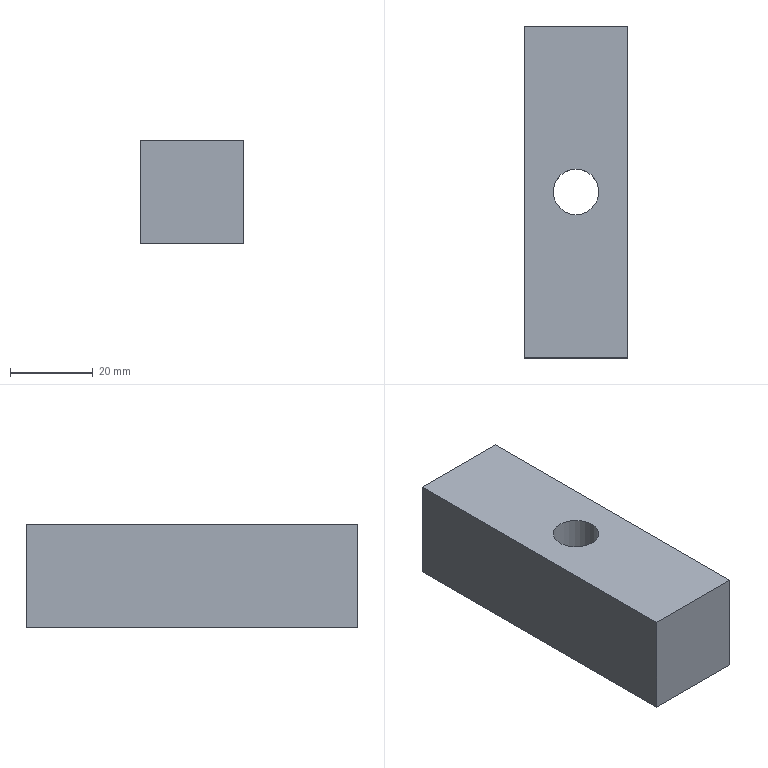Part | NX | features solid 2 | 1 solid | 9 faces | box 25 x 80 x 25 mm | volume 45711 mm3 | plane 7 | cylinder 2 | commonest cylinder face diameters 11 x1 18 x1
STEP:
#1=CARTESIAN_POINT('',(-317.5,-542.5,143.));
#2=VERTEX_POINT('',#1);
#3=CARTESIAN_POINT('',(-317.5,-542.5,118.));
#4=VERTEX_POINT('',#3);
#5=CARTESIAN_POINT('',(-317.5,-542.5,143.));
#6=DIRECTION('',(0.,0.,1.));
#7=VECTOR('',#6,1000.);
#8=LINE('',#5,#7);
#9=EDGE_CURVE('',#2,#4,#8,.F.);
#10=ORIENTED_EDGE('',*,*,#9,.T.);
#11=CARTESIAN_POINT('',(-292.5,-542.5,118.));
#12=VERTEX_POINT('',#11);
#13=CARTESIAN_POINT('',(-317.5,-542.5,118.));
#14=DIRECTION('',(1.,0.,0.));
#15=VECTOR('',#14,1000.);
#16=LINE('',#13,#15);
#17=EDGE_CURVE('',#4,#12,#16,.T.);
#18=ORIENTED_EDGE('',*,*,#17,.T.);
#19=CARTESIAN_POINT('',(-292.5,-542.5,143.));
#20=VERTEX_POINT('',#19);
#21=CARTESIAN_POINT('',(-292.5,-542.5,143.));
#22=DIRECTION('',(0.,0.,-1.));
#23=VECTOR('',#22,1000.);
#24=LINE('',#21,#23);
#25=EDGE_CURVE('',#20,#12,#24,.T.);
#26=ORIENTED_EDGE('',*,*,#25,.F.);
#27=CARTESIAN_POINT('',(-317.5,-542.5,143.));
#28=DIRECTION('',(1.,0.,0.));
#29=VECTOR('',#28,1000.);
#30=LINE('',#27,#29);
#31=EDGE_CURVE('',#2,#20,#30,.T.);
#32=ORIENTED_EDGE('',*,*,#31,.F.);
#33=EDGE_LOOP('',(#10,#18,#26,#32));
#34=FACE_BOUND('',#33,.T.);
#35=CARTESIAN_POINT('',(-317.5,-542.5,143.));
#36=DIRECTION('',(0.,-1.,0.));
#37=DIRECTION('',(1.,0.,0.));
#38=AXIS2_PLACEMENT_3D('',#35,#36,#37);
#39=PLANE('',#38);
#40=ADVANCED_FACE('',(#34),#39,.T.);
#41=ORIENTED_EDGE('',*,*,#25,.T.);
#42=CARTESIAN_POINT('',(-292.5,-462.5,118.));
#43=VERTEX_POINT('',#42);
#44=CARTESIAN_POINT('',(-292.5,-539.5,118.));
#45=DIRECTION('',(0.,-1.,0.));
#46=VECTOR('',#45,1000.);
#47=LINE('',#44,#46);
#48=EDGE_CURVE('',#12,#43,#47,.F.);
#49=ORIENTED_EDGE('',*,*,#48,.T.);
#50=CARTESIAN_POINT('',(-292.5,-462.5,143.));
#51=VERTEX_POINT('',#50);
#52=CARTESIAN_POINT('',(-292.5,-462.5,143.));
#53=DIRECTION('',(0.,0.,1.));
#54=VECTOR('',#53,1000.);
#55=LINE('',#52,#54);
#56=EDGE_CURVE('',#51,#43,#55,.F.);
#57=ORIENTED_EDGE('',*,*,#56,.F.);
#58=CARTESIAN_POINT('',(-292.5,-539.5,143.));
#59=DIRECTION('',(0.,1.,0.));
#60=VECTOR('',#59,1000.);
#61=LINE('',#58,#60);
#62=EDGE_CURVE('',#20,#51,#61,.T.);
#63=ORIENTED_EDGE('',*,*,#62,.F.);
#64=EDGE_LOOP('',(#41,#49,#57,#63));
#65=FACE_BOUND('',#64,.T.);
#66=CARTESIAN_POINT('',(-292.5,-539.5,143.));
#67=DIRECTION('',(1.,0.,0.));
#68=DIRECTION('',(0.,1.,0.));
#69=AXIS2_PLACEMENT_3D('',#66,#67,#68);
#70=PLANE('',#69);
#71=ADVANCED_FACE('',(#65),#70,.T.);
#72=ORIENTED_EDGE('',*,*,#56,.T.);
#73=CARTESIAN_POINT('',(-317.5,-462.5,118.));
#74=VERTEX_POINT('',#73);
#75=CARTESIAN_POINT('',(-317.5,-462.5,118.));
#76=DIRECTION('',(-1.,0.,0.));
#77=VECTOR('',#76,1000.);
#78=LINE('',#75,#77);
#79=EDGE_CURVE('',#74,#43,#78,.F.);
#80=ORIENTED_EDGE('',*,*,#79,.F.);
#81=CARTESIAN_POINT('',(-317.5,-462.5,143.));
#82=VERTEX_POINT('',#81);
#83=CARTESIAN_POINT('',(-317.5,-462.5,143.));
#84=DIRECTION('',(0.,0.,-1.));
#85=VECTOR('',#84,1000.);
#86=LINE('',#83,#85);
#87=EDGE_CURVE('',#82,#74,#86,.T.);
#88=ORIENTED_EDGE('',*,*,#87,.F.);
#89=CARTESIAN_POINT('',(-317.5,-462.5,143.));
#90=DIRECTION('',(-1.,0.,0.));
#91=VECTOR('',#90,1000.);
#92=LINE('',#89,#91);
#93=EDGE_CURVE('',#82,#51,#92,.F.);
#94=ORIENTED_EDGE('',*,*,#93,.T.);
#95=EDGE_LOOP('',(#72,#80,#88,#94));
#96=FACE_BOUND('',#95,.T.);
#97=CARTESIAN_POINT('',(-317.5,-462.5,143.));
#98=DIRECTION('',(0.,-1.,0.));
#99=DIRECTION('',(1.,0.,0.));
#100=AXIS2_PLACEMENT_3D('',#97,#98,#99);
#101=PLANE('',#100);
#102=ADVANCED_FACE('',(#96),#101,.F.);
#103=CARTESIAN_POINT('',(-317.5,-539.5,143.));
#104=DIRECTION('',(0.,1.,0.));
#105=VECTOR('',#104,1000.);
#106=LINE('',#103,#105);
#107=EDGE_CURVE('',#2,#82,#106,.T.);
#108=ORIENTED_EDGE('',*,*,#107,.T.);
#109=ORIENTED_EDGE('',*,*,#87,.T.);
#110=CARTESIAN_POINT('',(-317.5,-539.5,118.));
#111=DIRECTION('',(0.,-1.,0.));
#112=VECTOR('',#111,1000.);
#113=LINE('',#110,#112);
#114=EDGE_CURVE('',#4,#74,#113,.F.);
#115=ORIENTED_EDGE('',*,*,#114,.F.);
#116=ORIENTED_EDGE('',*,*,#9,.F.);
#117=EDGE_LOOP('',(#108,#109,#115,#116));
#118=FACE_BOUND('',#117,.T.);
#119=CARTESIAN_POINT('',(-317.5,-539.5,143.));
#120=DIRECTION('',(1.,0.,0.));
#121=DIRECTION('',(0.,1.,0.));
#122=AXIS2_PLACEMENT_3D('',#119,#120,#121);
#123=PLANE('',#122);
#124=ADVANCED_FACE('',(#118),#123,.F.);
#125=CARTESIAN_POINT('',(-305.,-493.5,118.));
#126=VERTEX_POINT('',#125);
#127=CARTESIAN_POINT('',(-305.,-502.5,118.));
#128=DIRECTION('',(0.,0.,-1.));
#129=DIRECTION('',(0.,1.,0.));
#130=AXIS2_PLACEMENT_3D('',#127,#128,#129);
#131=CIRCLE('',#130,9.);
#132=EDGE_CURVE('',#126,#126,#131,.T.);
#133=ORIENTED_EDGE('',*,*,#132,.F.);
#134=EDGE_LOOP('',(#133));
#135=FACE_BOUND('',#134,.T.);
#136=ORIENTED_EDGE('',*,*,#79,.T.);
#137=ORIENTED_EDGE('',*,*,#48,.F.);
#138=ORIENTED_EDGE('',*,*,#17,.F.);
#139=ORIENTED_EDGE('',*,*,#114,.T.);
#140=EDGE_LOOP('',(#136,#137,#138,#139));
#141=FACE_BOUND('',#140,.T.);
#142=CARTESIAN_POINT('',(-317.5,-539.5,118.));
#143=DIRECTION('',(0.,0.,-1.));
#144=DIRECTION('',(0.,-1.,0.));
#145=AXIS2_PLACEMENT_3D('',#142,#143,#144);
#146=PLANE('',#145);
#147=ADVANCED_FACE('',(#135,#141),#146,.T.);
#148=CARTESIAN_POINT('',(-305.,-508.,143.));
#149=VERTEX_POINT('',#148);
#150=CARTESIAN_POINT('',(-305.,-502.5,143.));
#151=DIRECTION('',(0.,0.,1.));
#152=DIRECTION('',(0.,-1.,0.));
#153=AXIS2_PLACEMENT_3D('',#150,#151,#152);
#154=CIRCLE('',#153,5.5);
#155=EDGE_CURVE('',#149,#149,#154,.T.);
#156=ORIENTED_EDGE('',*,*,#155,.F.);
#157=EDGE_LOOP('',(#156));
#158=FACE_BOUND('',#157,.T.);
#159=ORIENTED_EDGE('',*,*,#93,.F.);
#160=ORIENTED_EDGE('',*,*,#107,.F.);
#161=ORIENTED_EDGE('',*,*,#31,.T.);
#162=ORIENTED_EDGE('',*,*,#62,.T.);
#163=EDGE_LOOP('',(#159,#160,#161,#162));
#164=FACE_BOUND('',#163,.T.);
#165=CARTESIAN_POINT('',(-317.5,-539.5,143.));
#166=DIRECTION('',(0.,0.,-1.));
#167=DIRECTION('',(0.,-1.,0.));
#168=AXIS2_PLACEMENT_3D('',#165,#166,#167);
#169=PLANE('',#168);
#170=ADVANCED_FACE('',(#158,#164),#169,.F.);
#171=CARTESIAN_POINT('',(-305.,-497.,130.));
#172=VERTEX_POINT('',#171);
#173=CARTESIAN_POINT('',(-305.,-502.5,130.));
#174=DIRECTION('',(0.,0.,-1.));
#175=DIRECTION('',(0.,1.,0.));
#176=AXIS2_PLACEMENT_3D('',#173,#174,#175);
#177=CIRCLE('',#176,5.5);
#178=EDGE_CURVE('',#172,#172,#177,.T.);
#179=ORIENTED_EDGE('',*,*,#178,.T.);
#180=EDGE_LOOP('',(#179));
#181=FACE_BOUND('',#180,.T.);
#182=ORIENTED_EDGE('',*,*,#155,.T.);
#183=EDGE_LOOP('',(#182));
#184=FACE_BOUND('',#183,.T.);
#185=CARTESIAN_POINT('',(-305.,-502.5,168.));
#186=DIRECTION('',(0.,0.,1.));
#187=DIRECTION('',(0.,1.,0.));
#188=AXIS2_PLACEMENT_3D('',#185,#186,#187);
#189=CYLINDRICAL_SURFACE('',#188,5.5);
#190=ADVANCED_FACE('',(#181,#184),#189,.F.);
#191=ORIENTED_EDGE('',*,*,#178,.F.);
#192=EDGE_LOOP('',(#191));
#193=FACE_BOUND('',#192,.T.);
#194=CARTESIAN_POINT('',(-305.,-493.5,130.));
#195=VERTEX_POINT('',#194);
#196=CARTESIAN_POINT('',(-305.,-502.5,130.));
#197=DIRECTION('',(0.,0.,-1.));
#198=DIRECTION('',(0.,1.,0.));
#199=AXIS2_PLACEMENT_3D('',#196,#197,#198);
#200=CIRCLE('',#199,9.);
#201=EDGE_CURVE('',#195,#195,#200,.T.);
#202=ORIENTED_EDGE('',*,*,#201,.T.);
#203=EDGE_LOOP('',(#202));
#204=FACE_BOUND('',#203,.T.);
#205=CARTESIAN_POINT('',(-305.,-502.5,130.));
#206=DIRECTION('',(0.,0.,1.));
#207=DIRECTION('',(0.,1.,0.));
#208=AXIS2_PLACEMENT_3D('',#205,#206,#207);
#209=PLANE('',#208);
#210=ADVANCED_FACE('',(#193,#204),#209,.F.);
#211=ORIENTED_EDGE('',*,*,#201,.F.);
#212=EDGE_LOOP('',(#211));
#213=FACE_BOUND('',#212,.T.);
#214=ORIENTED_EDGE('',*,*,#132,.T.);
#215=EDGE_LOOP('',(#214));
#216=FACE_BOUND('',#215,.T.);
#217=CARTESIAN_POINT('',(-305.,-502.5,118.));
#218=DIRECTION('',(0.,0.,1.));
#219=DIRECTION('',(0.,1.,0.));
#220=AXIS2_PLACEMENT_3D('',#217,#218,#219);
#221=CYLINDRICAL_SURFACE('',#220,9.);
#222=ADVANCED_FACE('',(#213,#216),#221,.F.);
#223=CLOSED_SHELL('',(#40,#71,#102,#124,#147,#170,#190,#210,#222));
#224=MANIFOLD_SOLID_BREP('',#223);
#225=(LENGTH_UNIT()NAMED_UNIT(*)SI_UNIT(.MILLI.,.METRE.));
#226=UNCERTAINTY_MEASURE_WITH_UNIT(LENGTH_MEASURE(0.00001),#225,'','');
#227=(NAMED_UNIT(*)PLANE_ANGLE_UNIT()SI_UNIT($,.RADIAN.));
#228=(NAMED_UNIT(*)SI_UNIT($,.STERADIAN.)SOLID_ANGLE_UNIT());
#229=(GEOMETRIC_REPRESENTATION_CONTEXT(3)GLOBAL_UNCERTAINTY_ASSIGNED_CONTEXT((#226))GLOBAL_UNIT_ASSIGNED_CONTEXT((#225,#227,#228))REPRESENTATION_CONTEXT('',''));
#230=ADVANCED_BREP_SHAPE_REPRESENTATION('',(#224),#229);